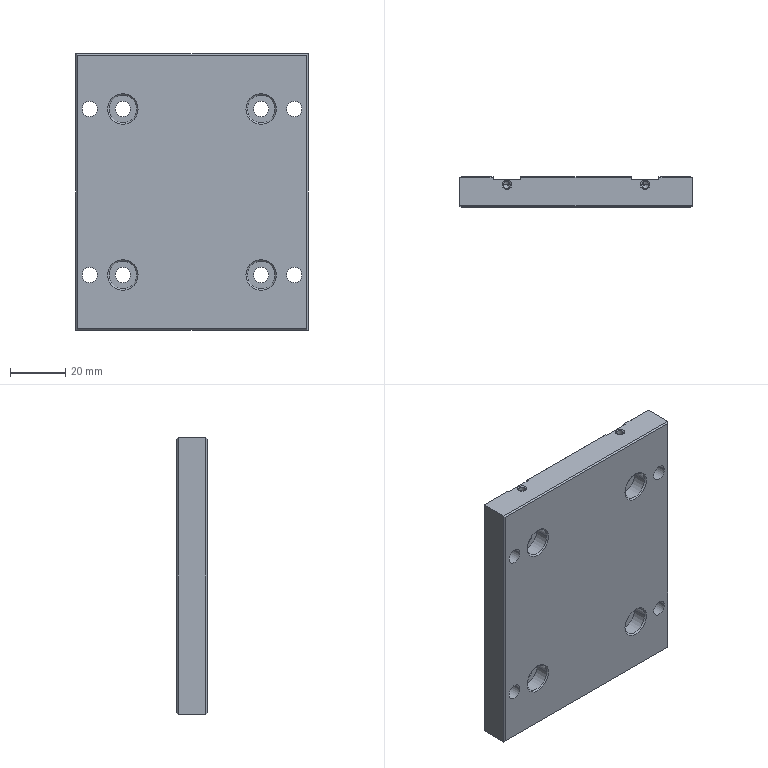Part | NX | 1 solid | 74 faces | box 84 x 11 x 100 mm | volume 87004 mm3 | plane 30 | cylinder 28 | cone 16 | commonest cylinder face diameters 5.5 x16 10 x8 2.5 x4